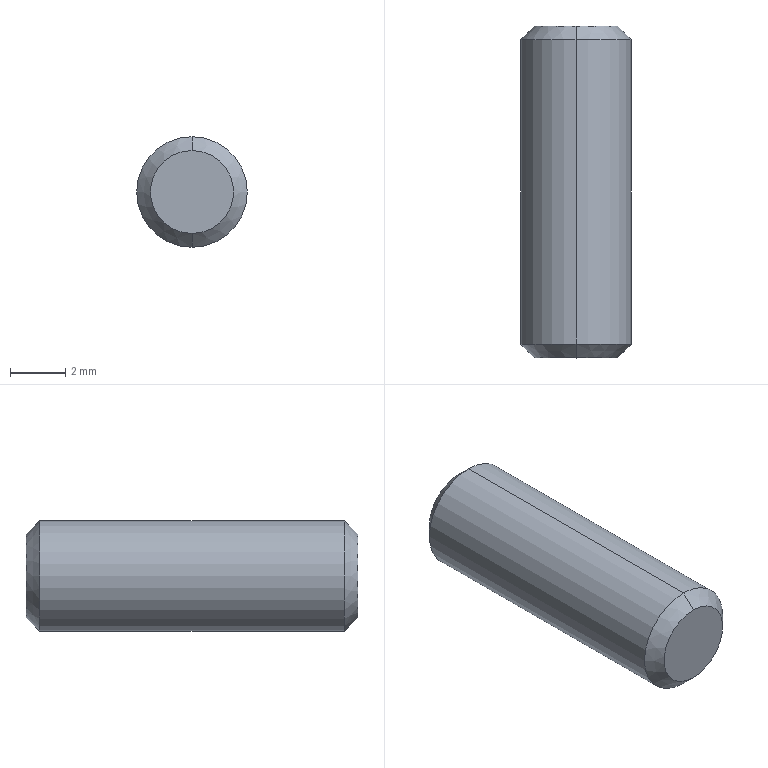Part | NX | features BREP 1 | 1 solid | 8 faces | box 4 x 12 x 4 mm | volume 147.917 mm3 | cone 4 | plane 2 | cylinder 2 | commonest cylinder face diameters 4 x2
STEP:
#1=CARTESIAN_POINT('',(0.,6.,1.5));
#2=VERTEX_POINT('',#1);
#3=CARTESIAN_POINT('',(0.,5.5,2.));
#4=VERTEX_POINT('',#3);
#5=CARTESIAN_POINT('',(0.,6.,1.5));
#6=DIRECTION('',(0.,-0.7071,0.7071));
#7=VECTOR('',#6,1000.);
#8=LINE('',#5,#7);
#9=EDGE_CURVE('',#2,#4,#8,.T.);
#10=ORIENTED_EDGE('',*,*,#9,.F.);
#11=CARTESIAN_POINT('',(0.,6.,-1.5));
#12=VERTEX_POINT('',#11);
#13=CARTESIAN_POINT('',(0.,6.,0.));
#14=DIRECTION('',(0.,1.,0.));
#15=DIRECTION('',(0.,0.,1.));
#16=AXIS2_PLACEMENT_3D('',#13,#14,#15);
#17=CIRCLE('',#16,1.5);
#18=EDGE_CURVE('',#12,#2,#17,.T.);
#19=ORIENTED_EDGE('',*,*,#18,.F.);
#20=CARTESIAN_POINT('',(0.,5.5,-2.));
#21=VERTEX_POINT('',#20);
#22=CARTESIAN_POINT('',(0.,6.,-1.5));
#23=DIRECTION('',(0.,-0.7071,-0.7071));
#24=VECTOR('',#23,1000.);
#25=LINE('',#22,#24);
#26=EDGE_CURVE('',#12,#21,#25,.T.);
#27=ORIENTED_EDGE('',*,*,#26,.T.);
#28=CARTESIAN_POINT('',(0.,5.5,0.));
#29=DIRECTION('',(0.,-1.,0.));
#30=DIRECTION('',(0.,0.,1.));
#31=AXIS2_PLACEMENT_3D('',#28,#29,#30);
#32=CIRCLE('',#31,2.);
#33=EDGE_CURVE('',#4,#21,#32,.T.);
#34=ORIENTED_EDGE('',*,*,#33,.F.);
#35=EDGE_LOOP('',(#10,#19,#27,#34));
#36=FACE_BOUND('',#35,.T.);
#37=CARTESIAN_POINT('',(0.,6.,0.));
#38=DIRECTION('',(0.,-1.,0.));
#39=DIRECTION('',(0.,0.,-1.));
#40=AXIS2_PLACEMENT_3D('',#37,#38,#39);
#41=CONICAL_SURFACE('',#40,1.5,0.7854);
#42=ADVANCED_FACE('',(#36),#41,.T.);
#43=CARTESIAN_POINT('',(0.,-5.5,-2.));
#44=VERTEX_POINT('',#43);
#45=CARTESIAN_POINT('',(0.,-6.,-1.5));
#46=VERTEX_POINT('',#45);
#47=CARTESIAN_POINT('',(0.,-5.5,-2.));
#48=DIRECTION('',(0.,0.7071,-0.7071));
#49=VECTOR('',#48,1000.);
#50=LINE('',#47,#49);
#51=EDGE_CURVE('',#44,#46,#50,.F.);
#52=ORIENTED_EDGE('',*,*,#51,.T.);
#53=CARTESIAN_POINT('',(0.,-6.,1.5));
#54=VERTEX_POINT('',#53);
#55=CARTESIAN_POINT('',(0.,-6.,0.));
#56=DIRECTION('',(0.,-1.,0.));
#57=DIRECTION('',(0.,0.,1.));
#58=AXIS2_PLACEMENT_3D('',#55,#56,#57);
#59=CIRCLE('',#58,1.5);
#60=EDGE_CURVE('',#54,#46,#59,.T.);
#61=ORIENTED_EDGE('',*,*,#60,.F.);
#62=CARTESIAN_POINT('',(0.,-5.5,2.));
#63=VERTEX_POINT('',#62);
#64=CARTESIAN_POINT('',(0.,-5.5,2.));
#65=DIRECTION('',(0.,0.7071,0.7071));
#66=VECTOR('',#65,1000.);
#67=LINE('',#64,#66);
#68=EDGE_CURVE('',#63,#54,#67,.F.);
#69=ORIENTED_EDGE('',*,*,#68,.F.);
#70=CARTESIAN_POINT('',(0.,-5.5,0.));
#71=DIRECTION('',(0.,1.,0.));
#72=DIRECTION('',(0.,0.,1.));
#73=AXIS2_PLACEMENT_3D('',#70,#71,#72);
#74=CIRCLE('',#73,2.);
#75=EDGE_CURVE('',#44,#63,#74,.T.);
#76=ORIENTED_EDGE('',*,*,#75,.F.);
#77=EDGE_LOOP('',(#52,#61,#69,#76));
#78=FACE_BOUND('',#77,.T.);
#79=CARTESIAN_POINT('',(0.,-5.5,0.));
#80=DIRECTION('',(0.,1.,0.));
#81=DIRECTION('',(0.,0.,1.));
#82=AXIS2_PLACEMENT_3D('',#79,#80,#81);
#83=CONICAL_SURFACE('',#82,2.,0.7854);
#84=ADVANCED_FACE('',(#78),#83,.T.);
#85=ORIENTED_EDGE('',*,*,#60,.T.);
#86=CARTESIAN_POINT('',(0.,-6.,0.));
#87=DIRECTION('',(0.,-1.,0.));
#88=DIRECTION('',(0.,0.,1.));
#89=AXIS2_PLACEMENT_3D('',#86,#87,#88);
#90=CIRCLE('',#89,1.5);
#91=EDGE_CURVE('',#46,#54,#90,.T.);
#92=ORIENTED_EDGE('',*,*,#91,.T.);
#93=EDGE_LOOP('',(#85,#92));
#94=FACE_BOUND('',#93,.T.);
#95=CARTESIAN_POINT('',(0.,-6.,0.));
#96=DIRECTION('',(0.,1.,0.));
#97=DIRECTION('',(0.,0.,1.));
#98=AXIS2_PLACEMENT_3D('',#95,#96,#97);
#99=PLANE('',#98);
#100=ADVANCED_FACE('',(#94),#99,.F.);
#101=ORIENTED_EDGE('',*,*,#18,.T.);
#102=CARTESIAN_POINT('',(0.,6.,0.));
#103=DIRECTION('',(0.,1.,0.));
#104=DIRECTION('',(0.,0.,1.));
#105=AXIS2_PLACEMENT_3D('',#102,#103,#104);
#106=CIRCLE('',#105,1.5);
#107=EDGE_CURVE('',#2,#12,#106,.T.);
#108=ORIENTED_EDGE('',*,*,#107,.T.);
#109=EDGE_LOOP('',(#101,#108));
#110=FACE_BOUND('',#109,.T.);
#111=CARTESIAN_POINT('',(0.,6.,0.));
#112=DIRECTION('',(0.,1.,0.));
#113=DIRECTION('',(0.,0.,1.));
#114=AXIS2_PLACEMENT_3D('',#111,#112,#113);
#115=PLANE('',#114);
#116=ADVANCED_FACE('',(#110),#115,.T.);
#117=CARTESIAN_POINT('',(0.,6.,2.));
#118=DIRECTION('',(0.,-1.,0.));
#119=VECTOR('',#118,1000.);
#120=LINE('',#117,#119);
#121=EDGE_CURVE('',#4,#63,#120,.T.);
#122=ORIENTED_EDGE('',*,*,#121,.F.);
#123=ORIENTED_EDGE('',*,*,#33,.T.);
#124=CARTESIAN_POINT('',(0.,6.,-2.));
#125=DIRECTION('',(0.,-1.,0.));
#126=VECTOR('',#125,1000.);
#127=LINE('',#124,#126);
#128=EDGE_CURVE('',#21,#44,#127,.T.);
#129=ORIENTED_EDGE('',*,*,#128,.T.);
#130=ORIENTED_EDGE('',*,*,#75,.T.);
#131=EDGE_LOOP('',(#122,#123,#129,#130));
#132=FACE_BOUND('',#131,.T.);
#133=CARTESIAN_POINT('',(0.,6.,0.));
#134=DIRECTION('',(0.,-1.,0.));
#135=DIRECTION('',(0.,0.,-1.));
#136=AXIS2_PLACEMENT_3D('',#133,#134,#135);
#137=CYLINDRICAL_SURFACE('',#136,2.);
#138=ADVANCED_FACE('',(#132),#137,.T.);
#139=CARTESIAN_POINT('',(0.,5.5,0.));
#140=DIRECTION('',(0.,-1.,0.));
#141=DIRECTION('',(0.,0.,1.));
#142=AXIS2_PLACEMENT_3D('',#139,#140,#141);
#143=CIRCLE('',#142,2.);
#144=EDGE_CURVE('',#21,#4,#143,.T.);
#145=ORIENTED_EDGE('',*,*,#144,.T.);
#146=ORIENTED_EDGE('',*,*,#121,.T.);
#147=CARTESIAN_POINT('',(0.,-5.5,0.));
#148=DIRECTION('',(0.,1.,0.));
#149=DIRECTION('',(0.,0.,1.));
#150=AXIS2_PLACEMENT_3D('',#147,#148,#149);
#151=CIRCLE('',#150,2.);
#152=EDGE_CURVE('',#63,#44,#151,.T.);
#153=ORIENTED_EDGE('',*,*,#152,.T.);
#154=ORIENTED_EDGE('',*,*,#128,.F.);
#155=EDGE_LOOP('',(#145,#146,#153,#154));
#156=FACE_BOUND('',#155,.T.);
#157=CARTESIAN_POINT('',(0.,6.,0.));
#158=DIRECTION('',(0.,-1.,0.));
#159=DIRECTION('',(0.,0.,-1.));
#160=AXIS2_PLACEMENT_3D('',#157,#158,#159);
#161=CYLINDRICAL_SURFACE('',#160,2.);
#162=ADVANCED_FACE('',(#156),#161,.T.);
#163=ORIENTED_EDGE('',*,*,#91,.F.);
#164=ORIENTED_EDGE('',*,*,#51,.F.);
#165=ORIENTED_EDGE('',*,*,#152,.F.);
#166=ORIENTED_EDGE('',*,*,#68,.T.);
#167=EDGE_LOOP('',(#163,#164,#165,#166));
#168=FACE_BOUND('',#167,.T.);
#169=CARTESIAN_POINT('',(0.,-5.5,0.));
#170=DIRECTION('',(0.,1.,0.));
#171=DIRECTION('',(0.,0.,1.));
#172=AXIS2_PLACEMENT_3D('',#169,#170,#171);
#173=CONICAL_SURFACE('',#172,2.,0.7854);
#174=ADVANCED_FACE('',(#168),#173,.T.);
#175=ORIENTED_EDGE('',*,*,#107,.F.);
#176=ORIENTED_EDGE('',*,*,#9,.T.);
#177=ORIENTED_EDGE('',*,*,#144,.F.);
#178=ORIENTED_EDGE('',*,*,#26,.F.);
#179=EDGE_LOOP('',(#175,#176,#177,#178));
#180=FACE_BOUND('',#179,.T.);
#181=CARTESIAN_POINT('',(0.,6.,0.));
#182=DIRECTION('',(0.,-1.,0.));
#183=DIRECTION('',(0.,0.,-1.));
#184=AXIS2_PLACEMENT_3D('',#181,#182,#183);
#185=CONICAL_SURFACE('',#184,1.5,0.7854);
#186=ADVANCED_FACE('',(#180),#185,.T.);
#187=CLOSED_SHELL('',(#42,#84,#100,#116,#138,#162,#174,#186));
#188=MANIFOLD_SOLID_BREP('',#187);
#189=(LENGTH_UNIT()NAMED_UNIT(*)SI_UNIT(.MILLI.,.METRE.));
#190=UNCERTAINTY_MEASURE_WITH_UNIT(LENGTH_MEASURE(0.00001),#189,'','');
#191=(NAMED_UNIT(*)PLANE_ANGLE_UNIT()SI_UNIT($,.RADIAN.));
#192=(NAMED_UNIT(*)SI_UNIT($,.STERADIAN.)SOLID_ANGLE_UNIT());
#193=(GEOMETRIC_REPRESENTATION_CONTEXT(3)GLOBAL_UNCERTAINTY_ASSIGNED_CONTEXT((#190))GLOBAL_UNIT_ASSIGNED_CONTEXT((#189,#191,#192))REPRESENTATION_CONTEXT('',''));
#194=ADVANCED_BREP_SHAPE_REPRESENTATION('',(#188),#193);